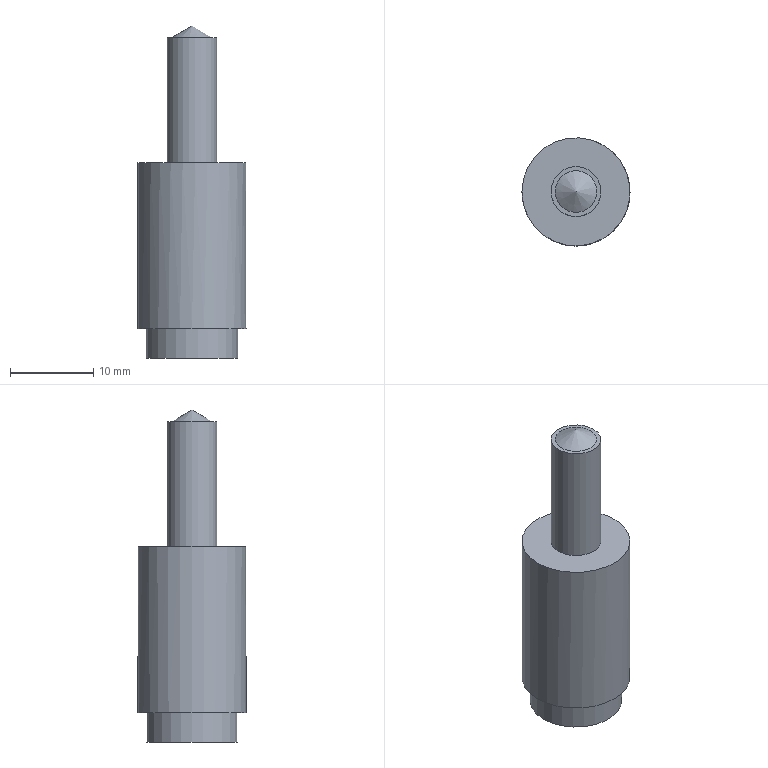Part | STEP file | KBQ13.00 | 1 solid | 15 faces | box 13 x 13 x 39.94 mm | volume 3312 mm3 | plane 11 | cylinder 3 | cone 1 | commonest cylinder face diameters 6 x1 11 x1 13 x1